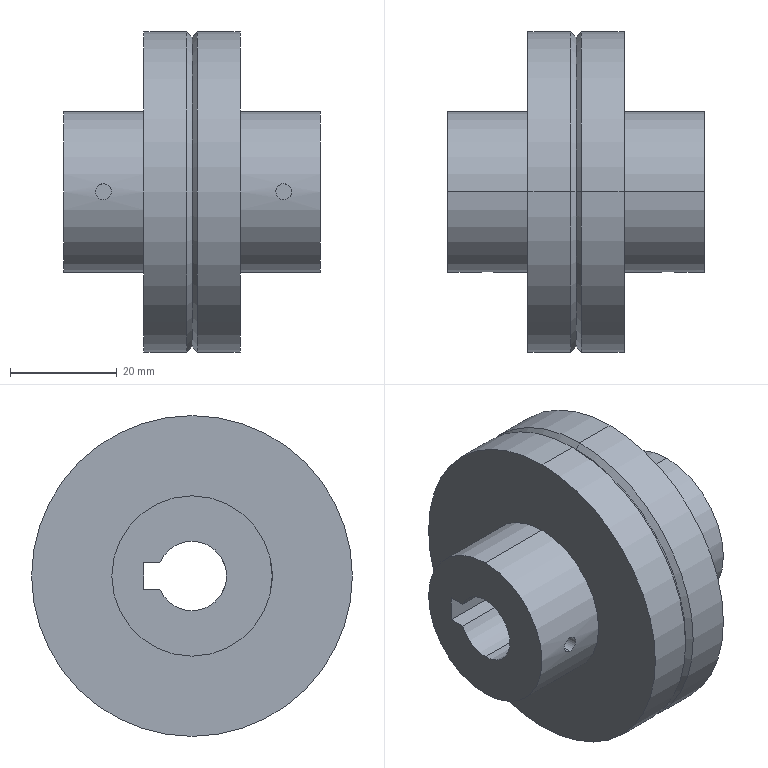Part | NX | features BREP 1 | 1 solid | 32 faces | box 48 x 60 x 60 mm | volume 63736 mm3 | cylinder 18 | plane 10 | cone 4 | commonest cylinder face diameters 3 x4 30 x4 60 x4 13 x3 15 x3
STEP:
#1=CARTESIAN_POINT('',(7.432,-6.331,-1.474));
#2=VERTEX_POINT('',#1);
#3=CARTESIAN_POINT('',(7.432,-6.318,1.526));
#4=VERTEX_POINT('',#3);
#5=CARTESIAN_POINT('',(7.432,-6.331,-1.474));
#6=CARTESIAN_POINT('',(7.034,-6.331,-1.474));
#7=CARTESIAN_POINT('',(6.259,-6.418,-1.149));
#8=CARTESIAN_POINT('',(5.768,-6.543,0.02457));
#9=CARTESIAN_POINT('',(6.259,-6.409,1.201));
#10=CARTESIAN_POINT('',(7.034,-6.318,1.526));
#11=CARTESIAN_POINT('',(7.432,-6.318,1.526));
#12=B_SPLINE_CURVE_WITH_KNOTS('',3,(#5,#6,#7,#8,#9,#10,#11),.UNSPECIFIED.,.F.,.F.,(4,1,1,1,4),(0.,0.001176,0.002352,0.003528,0.004704),.UNSPECIFIED.);
#13=EDGE_CURVE('',#2,#4,#12,.T.);
#14=ORIENTED_EDGE('',*,*,#13,.T.);
#15=CARTESIAN_POINT('',(7.432,-14.919,1.561));
#16=VERTEX_POINT('',#15);
#17=CARTESIAN_POINT('',(7.432,-14.994,1.561));
#18=DIRECTION('',(0.,-1.,0.004061));
#19=VECTOR('',#18,1000.);
#20=LINE('',#17,#19);
#21=EDGE_CURVE('',#16,#4,#20,.F.);
#22=ORIENTED_EDGE('',*,*,#21,.F.);
#23=CARTESIAN_POINT('',(7.432,-14.931,-1.439));
#24=VERTEX_POINT('',#23);
#25=CARTESIAN_POINT('',(7.432,-14.919,1.561));
#26=CARTESIAN_POINT('',(7.035,-14.919,1.561));
#27=CARTESIAN_POINT('',(6.259,-14.958,1.236));
#28=CARTESIAN_POINT('',(5.769,-15.019,0.0625));
#29=CARTESIAN_POINT('',(6.258,-14.967,-1.114));
#30=CARTESIAN_POINT('',(7.035,-14.931,-1.439));
#31=CARTESIAN_POINT('',(7.432,-14.931,-1.439));
#32=B_SPLINE_CURVE_WITH_KNOTS('',3,(#25,#26,#27,#28,#29,#30,#31),.UNSPECIFIED.,.F.,.F.,(4,1,1,1,4),(0.,0.001173,0.002346,0.003519,0.004692),.UNSPECIFIED.);
#33=EDGE_CURVE('',#16,#24,#32,.T.);
#34=ORIENTED_EDGE('',*,*,#33,.T.);
#35=CARTESIAN_POINT('',(7.432,-15.006,-1.439));
#36=DIRECTION('',(0.,-1.,0.004061));
#37=VECTOR('',#36,1000.);
#38=LINE('',#35,#37);
#39=EDGE_CURVE('',#24,#2,#38,.F.);
#40=ORIENTED_EDGE('',*,*,#39,.T.);
#41=EDGE_LOOP('',(#14,#22,#34,#40));
#42=FACE_BOUND('',#41,.T.);
#43=CARTESIAN_POINT('',(7.432,-15.,0.06091));
#44=DIRECTION('',(0.,-1.,0.004061));
#45=DIRECTION('',(0.,0.004061,1.));
#46=AXIS2_PLACEMENT_3D('',#43,#44,#45);
#47=CYLINDRICAL_SURFACE('',#46,1.5);
#48=ADVANCED_FACE('',(#42),#47,.F.);
#49=CARTESIAN_POINT('',(41.177,-7.354,-1.47));
#50=VERTEX_POINT('',#49);
#51=CARTESIAN_POINT('',(41.177,-7.342,1.53));
#52=VERTEX_POINT('',#51);
#53=CARTESIAN_POINT('',(41.177,-7.354,-1.47));
#54=CARTESIAN_POINT('',(40.78,-7.354,-1.47));
#55=CARTESIAN_POINT('',(40.004,-7.43,-1.145));
#56=CARTESIAN_POINT('',(39.514,-7.537,0.02875));
#57=CARTESIAN_POINT('',(40.003,-7.42,1.205));
#58=CARTESIAN_POINT('',(40.78,-7.342,1.53));
#59=CARTESIAN_POINT('',(41.177,-7.342,1.53));
#60=B_SPLINE_CURVE_WITH_KNOTS('',3,(#53,#54,#55,#56,#57,#58,#59),.UNSPECIFIED.,.F.,.F.,(4,1,1,1,4),(0.,0.001175,0.00235,0.003525,0.0047),.UNSPECIFIED.);
#61=EDGE_CURVE('',#50,#52,#60,.T.);
#62=ORIENTED_EDGE('',*,*,#61,.T.);
#63=CARTESIAN_POINT('',(41.177,-14.919,1.561));
#64=VERTEX_POINT('',#63);
#65=CARTESIAN_POINT('',(41.177,-14.994,1.561));
#66=DIRECTION('',(0.,-1.,0.004061));
#67=VECTOR('',#66,1000.);
#68=LINE('',#65,#67);
#69=EDGE_CURVE('',#64,#52,#68,.F.);
#70=ORIENTED_EDGE('',*,*,#69,.F.);
#71=CARTESIAN_POINT('',(41.177,-14.931,-1.439));
#72=VERTEX_POINT('',#71);
#73=CARTESIAN_POINT('',(41.177,-14.919,1.561));
#74=CARTESIAN_POINT('',(40.781,-14.919,1.561));
#75=CARTESIAN_POINT('',(40.004,-14.958,1.236));
#76=CARTESIAN_POINT('',(39.514,-15.019,0.0625));
#77=CARTESIAN_POINT('',(40.003,-14.967,-1.114));
#78=CARTESIAN_POINT('',(40.781,-14.931,-1.439));
#79=CARTESIAN_POINT('',(41.177,-14.931,-1.439));
#80=B_SPLINE_CURVE_WITH_KNOTS('',3,(#73,#74,#75,#76,#77,#78,#79),.UNSPECIFIED.,.F.,.F.,(4,1,1,1,4),(0.,0.001173,0.002346,0.003519,0.004692),.UNSPECIFIED.);
#81=EDGE_CURVE('',#64,#72,#80,.T.);
#82=ORIENTED_EDGE('',*,*,#81,.T.);
#83=CARTESIAN_POINT('',(41.177,-15.006,-1.439));
#84=DIRECTION('',(0.,-1.,0.004061));
#85=VECTOR('',#84,1000.);
#86=LINE('',#83,#85);
#87=EDGE_CURVE('',#72,#50,#86,.F.);
#88=ORIENTED_EDGE('',*,*,#87,.T.);
#89=EDGE_LOOP('',(#62,#70,#82,#88));
#90=FACE_BOUND('',#89,.T.);
#91=CARTESIAN_POINT('',(41.177,-15.,0.06091));
#92=DIRECTION('',(0.,-1.,0.004061));
#93=DIRECTION('',(0.,0.004061,1.));
#94=AXIS2_PLACEMENT_3D('',#91,#92,#93);
#95=CYLINDRICAL_SURFACE('',#94,1.5);
#96=ADVANCED_FACE('',(#90),#95,.F.);
#97=CARTESIAN_POINT('',(24.,0.,29.));
#98=VERTEX_POINT('',#97);
#99=CARTESIAN_POINT('',(24.,0.,-29.));
#100=VERTEX_POINT('',#99);
#101=CARTESIAN_POINT('',(24.,0.,0.));
#102=DIRECTION('',(-1.,0.,0.));
#103=DIRECTION('',(0.,0.,1.));
#104=AXIS2_PLACEMENT_3D('',#101,#102,#103);
#105=CIRCLE('',#104,29.);
#106=EDGE_CURVE('',#98,#100,#105,.T.);
#107=ORIENTED_EDGE('',*,*,#106,.F.);
#108=CARTESIAN_POINT('',(25.,0.,30.));
#109=VERTEX_POINT('',#108);
#110=CARTESIAN_POINT('',(24.,0.,29.));
#111=DIRECTION('',(0.7071,0.,0.7071));
#112=VECTOR('',#111,1000.);
#113=LINE('',#110,#112);
#114=EDGE_CURVE('',#109,#98,#113,.F.);
#115=ORIENTED_EDGE('',*,*,#114,.F.);
#116=CARTESIAN_POINT('',(25.,0.,-30.));
#117=VERTEX_POINT('',#116);
#118=CARTESIAN_POINT('',(25.,0.,0.));
#119=DIRECTION('',(-1.,0.,0.));
#120=DIRECTION('',(0.,0.,1.));
#121=AXIS2_PLACEMENT_3D('',#118,#119,#120);
#122=CIRCLE('',#121,30.);
#123=EDGE_CURVE('',#109,#117,#122,.T.);
#124=ORIENTED_EDGE('',*,*,#123,.T.);
#125=CARTESIAN_POINT('',(24.,0.,-29.));
#126=DIRECTION('',(0.7071,0.,-0.7071));
#127=VECTOR('',#126,1000.);
#128=LINE('',#125,#127);
#129=EDGE_CURVE('',#117,#100,#128,.F.);
#130=ORIENTED_EDGE('',*,*,#129,.T.);
#131=EDGE_LOOP('',(#107,#115,#124,#130));
#132=FACE_BOUND('',#131,.T.);
#133=CARTESIAN_POINT('',(24.,0.,0.));
#134=DIRECTION('',(1.,0.,0.));
#135=DIRECTION('',(0.,0.,1.));
#136=AXIS2_PLACEMENT_3D('',#133,#134,#135);
#137=CONICAL_SURFACE('',#136,29.,0.7854);
#138=ADVANCED_FACE('',(#132),#137,.T.);
#139=CARTESIAN_POINT('',(33.,0.,30.));
#140=VERTEX_POINT('',#139);
#141=CARTESIAN_POINT('',(33.,0.,-30.));
#142=VERTEX_POINT('',#141);
#143=CARTESIAN_POINT('',(33.,0.,0.));
#144=DIRECTION('',(-1.,0.,0.));
#145=DIRECTION('',(0.,0.,1.));
#146=AXIS2_PLACEMENT_3D('',#143,#144,#145);
#147=CIRCLE('',#146,30.);
#148=EDGE_CURVE('',#140,#142,#147,.T.);
#149=ORIENTED_EDGE('',*,*,#148,.T.);
#150=CARTESIAN_POINT('',(0.,0.,-30.));
#151=DIRECTION('',(-1.,0.,0.));
#152=VECTOR('',#151,1000.);
#153=LINE('',#150,#152);
#154=EDGE_CURVE('',#142,#117,#153,.T.);
#155=ORIENTED_EDGE('',*,*,#154,.T.);
#156=ORIENTED_EDGE('',*,*,#123,.F.);
#157=CARTESIAN_POINT('',(0.,0.,30.));
#158=DIRECTION('',(-1.,0.,0.));
#159=VECTOR('',#158,1000.);
#160=LINE('',#157,#159);
#161=EDGE_CURVE('',#140,#109,#160,.T.);
#162=ORIENTED_EDGE('',*,*,#161,.F.);
#163=EDGE_LOOP('',(#149,#155,#156,#162));
#164=FACE_BOUND('',#163,.T.);
#165=CARTESIAN_POINT('',(0.,0.,0.));
#166=DIRECTION('',(-1.,0.,0.));
#167=DIRECTION('',(0.,0.,-1.));
#168=AXIS2_PLACEMENT_3D('',#165,#166,#167);
#169=CYLINDRICAL_SURFACE('',#168,30.);
#170=ADVANCED_FACE('',(#164),#169,.T.);
#171=CARTESIAN_POINT('',(48.,0.,15.));
#172=VERTEX_POINT('',#171);
#173=CARTESIAN_POINT('',(48.,0.,-15.));
#174=VERTEX_POINT('',#173);
#175=CARTESIAN_POINT('',(48.,0.,0.));
#176=DIRECTION('',(-1.,0.,0.));
#177=DIRECTION('',(0.,0.,1.));
#178=AXIS2_PLACEMENT_3D('',#175,#176,#177);
#179=CIRCLE('',#178,15.);
#180=EDGE_CURVE('',#172,#174,#179,.T.);
#181=ORIENTED_EDGE('',*,*,#180,.T.);
#182=CARTESIAN_POINT('',(33.,0.,-15.));
#183=VERTEX_POINT('',#182);
#184=CARTESIAN_POINT('',(0.,0.,-15.));
#185=DIRECTION('',(-1.,0.,0.));
#186=VECTOR('',#185,1000.);
#187=LINE('',#184,#186);
#188=EDGE_CURVE('',#174,#183,#187,.T.);
#189=ORIENTED_EDGE('',*,*,#188,.T.);
#190=CARTESIAN_POINT('',(33.,0.,15.));
#191=VERTEX_POINT('',#190);
#192=CARTESIAN_POINT('',(33.,0.,0.));
#193=DIRECTION('',(-1.,0.,0.));
#194=DIRECTION('',(0.,0.,1.));
#195=AXIS2_PLACEMENT_3D('',#192,#193,#194);
#196=CIRCLE('',#195,15.);
#197=EDGE_CURVE('',#191,#183,#196,.T.);
#198=ORIENTED_EDGE('',*,*,#197,.F.);
#199=CARTESIAN_POINT('',(0.,0.,15.));
#200=DIRECTION('',(-1.,0.,0.));
#201=VECTOR('',#200,1000.);
#202=LINE('',#199,#201);
#203=EDGE_CURVE('',#172,#191,#202,.T.);
#204=ORIENTED_EDGE('',*,*,#203,.F.);
#205=EDGE_LOOP('',(#181,#189,#198,#204));
#206=FACE_BOUND('',#205,.T.);
#207=CARTESIAN_POINT('',(0.,0.,0.));
#208=DIRECTION('',(-1.,0.,0.));
#209=DIRECTION('',(0.,0.,-1.));
#210=AXIS2_PLACEMENT_3D('',#207,#208,#209);
#211=CYLINDRICAL_SURFACE('',#210,15.);
#212=ADVANCED_FACE('',(#206),#211,.T.);
#213=CARTESIAN_POINT('',(48.,0.,-7.5));
#214=VERTEX_POINT('',#213);
#215=CARTESIAN_POINT('',(48.,0.,7.5));
#216=VERTEX_POINT('',#215);
#217=CARTESIAN_POINT('',(48.,0.,0.));
#218=DIRECTION('',(-1.,0.,0.));
#219=DIRECTION('',(0.,0.,1.));
#220=AXIS2_PLACEMENT_3D('',#217,#218,#219);
#221=CIRCLE('',#220,7.5);
#222=EDGE_CURVE('',#214,#216,#221,.T.);
#223=ORIENTED_EDGE('',*,*,#222,.F.);
#224=CARTESIAN_POINT('',(24.,0.,-7.5));
#225=VERTEX_POINT('',#224);
#226=CARTESIAN_POINT('',(0.,0.,-7.5));
#227=DIRECTION('',(-1.,0.,0.));
#228=VECTOR('',#227,1000.);
#229=LINE('',#226,#228);
#230=EDGE_CURVE('',#214,#225,#229,.T.);
#231=ORIENTED_EDGE('',*,*,#230,.T.);
#232=CARTESIAN_POINT('',(24.,0.,7.5));
#233=VERTEX_POINT('',#232);
#234=CARTESIAN_POINT('',(24.,0.,0.));
#235=DIRECTION('',(-1.,0.,0.));
#236=DIRECTION('',(0.,0.,1.));
#237=AXIS2_PLACEMENT_3D('',#234,#235,#236);
#238=CIRCLE('',#237,7.5);
#239=EDGE_CURVE('',#225,#233,#238,.T.);
#240=ORIENTED_EDGE('',*,*,#239,.T.);
#241=CARTESIAN_POINT('',(0.,0.,7.5));
#242=DIRECTION('',(-1.,0.,0.));
#243=VECTOR('',#242,1000.);
#244=LINE('',#241,#243);
#245=EDGE_CURVE('',#216,#233,#244,.T.);
#246=ORIENTED_EDGE('',*,*,#245,.F.);
#247=EDGE_LOOP('',(#223,#231,#240,#246));
#248=FACE_BOUND('',#247,.T.);
#249=ORIENTED_EDGE('',*,*,#61,.F.);
#250=CARTESIAN_POINT('',(41.177,-7.342,1.53));
#251=CARTESIAN_POINT('',(41.575,-7.342,1.53));
#252=CARTESIAN_POINT('',(42.35,-7.42,1.205));
#253=CARTESIAN_POINT('',(42.841,-7.537,0.03247));
#254=CARTESIAN_POINT('',(42.351,-7.43,-1.145));
#255=CARTESIAN_POINT('',(41.575,-7.354,-1.47));
#256=CARTESIAN_POINT('',(41.177,-7.354,-1.47));
#257=B_SPLINE_CURVE_WITH_KNOTS('',3,(#250,#251,#252,#253,#254,#255,#256),.UNSPECIFIED.,.F.,.F.,(4,1,1,1,4),(0.,0.001175,0.00235,0.003525,0.0047),.UNSPECIFIED.);
#258=EDGE_CURVE('',#52,#50,#257,.T.);
#259=ORIENTED_EDGE('',*,*,#258,.F.);
#260=EDGE_LOOP('',(#249,#259));
#261=FACE_BOUND('',#260,.T.);
#262=CARTESIAN_POINT('',(0.,0.,0.));
#263=DIRECTION('',(-1.,0.,0.));
#264=DIRECTION('',(0.,0.,-1.));
#265=AXIS2_PLACEMENT_3D('',#262,#263,#264);
#266=CYLINDRICAL_SURFACE('',#265,7.5);
#267=ADVANCED_FACE('',(#248,#261),#266,.F.);
#268=CARTESIAN_POINT('',(48.,7.071,2.5));
#269=VERTEX_POINT('',#268);
#270=CARTESIAN_POINT('',(48.,0.,0.));
#271=DIRECTION('',(-1.,0.,0.));
#272=DIRECTION('',(0.,0.,1.));
#273=AXIS2_PLACEMENT_3D('',#270,#271,#272);
#274=CIRCLE('',#273,7.5);
#275=EDGE_CURVE('',#216,#269,#274,.T.);
#276=ORIENTED_EDGE('',*,*,#275,.F.);
#277=ORIENTED_EDGE('',*,*,#245,.T.);
#278=CARTESIAN_POINT('',(24.,7.071,2.5));
#279=VERTEX_POINT('',#278);
#280=CARTESIAN_POINT('',(24.,0.,0.));
#281=DIRECTION('',(-1.,0.,0.));
#282=DIRECTION('',(0.,0.,1.));
#283=AXIS2_PLACEMENT_3D('',#280,#281,#282);
#284=CIRCLE('',#283,7.5);
#285=EDGE_CURVE('',#233,#279,#284,.T.);
#286=ORIENTED_EDGE('',*,*,#285,.T.);
#287=CARTESIAN_POINT('',(24.,7.071,2.5));
#288=DIRECTION('',(1.,0.,0.));
#289=VECTOR('',#288,1000.);
#290=LINE('',#287,#289);
#291=EDGE_CURVE('',#279,#269,#290,.T.);
#292=ORIENTED_EDGE('',*,*,#291,.T.);
#293=EDGE_LOOP('',(#276,#277,#286,#292));
#294=FACE_BOUND('',#293,.T.);
#295=CARTESIAN_POINT('',(0.,0.,0.));
#296=DIRECTION('',(-1.,0.,0.));
#297=DIRECTION('',(0.,0.,-1.));
#298=AXIS2_PLACEMENT_3D('',#295,#296,#297);
#299=CYLINDRICAL_SURFACE('',#298,7.5);
#300=ADVANCED_FACE('',(#294),#299,.F.);
#301=CARTESIAN_POINT('',(24.,0.,-6.5));
#302=VERTEX_POINT('',#301);
#303=CARTESIAN_POINT('',(24.,0.,6.5));
#304=VERTEX_POINT('',#303);
#305=CARTESIAN_POINT('',(24.,0.,0.));
#306=DIRECTION('',(-1.,0.,0.));
#307=DIRECTION('',(0.,0.,1.));
#308=AXIS2_PLACEMENT_3D('',#305,#306,#307);
#309=CIRCLE('',#308,6.5);
#310=EDGE_CURVE('',#302,#304,#309,.T.);
#311=ORIENTED_EDGE('',*,*,#310,.F.);
#312=CARTESIAN_POINT('',(0.,0.,-6.5));
#313=VERTEX_POINT('',#312);
#314=CARTESIAN_POINT('',(0.,0.,-6.5));
#315=DIRECTION('',(-1.,0.,0.));
#316=VECTOR('',#315,1000.);
#317=LINE('',#314,#316);
#318=EDGE_CURVE('',#302,#313,#317,.T.);
#319=ORIENTED_EDGE('',*,*,#318,.T.);
#320=CARTESIAN_POINT('',(0.,0.,6.5));
#321=VERTEX_POINT('',#320);
#322=CARTESIAN_POINT('',(0.,0.,0.));
#323=DIRECTION('',(-1.,0.,0.));
#324=DIRECTION('',(0.,0.,1.));
#325=AXIS2_PLACEMENT_3D('',#322,#323,#324);
#326=CIRCLE('',#325,6.5);
#327=EDGE_CURVE('',#313,#321,#326,.T.);
#328=ORIENTED_EDGE('',*,*,#327,.T.);
#329=CARTESIAN_POINT('',(0.,0.,6.5));
#330=DIRECTION('',(-1.,0.,0.));
#331=VECTOR('',#330,1000.);
#332=LINE('',#329,#331);
#333=EDGE_CURVE('',#304,#321,#332,.T.);
#334=ORIENTED_EDGE('',*,*,#333,.F.);
#335=EDGE_LOOP('',(#311,#319,#328,#334));
#336=FACE_BOUND('',#335,.T.);
#337=ORIENTED_EDGE('',*,*,#13,.F.);
#338=CARTESIAN_POINT('',(7.432,-6.318,1.526));
#339=CARTESIAN_POINT('',(7.83,-6.318,1.526));
#340=CARTESIAN_POINT('',(8.604,-6.409,1.201));
#341=CARTESIAN_POINT('',(9.096,-6.543,0.02857));
#342=CARTESIAN_POINT('',(8.605,-6.418,-1.149));
#343=CARTESIAN_POINT('',(7.83,-6.331,-1.474));
#344=CARTESIAN_POINT('',(7.432,-6.331,-1.474));
#345=B_SPLINE_CURVE_WITH_KNOTS('',3,(#338,#339,#340,#341,#342,#343,#344),.UNSPECIFIED.,.F.,.F.,(4,1,1,1,4),(0.,0.001176,0.002352,0.003528,0.004704),.UNSPECIFIED.);
#346=EDGE_CURVE('',#4,#2,#345,.T.);
#347=ORIENTED_EDGE('',*,*,#346,.F.);
#348=EDGE_LOOP('',(#337,#347));
#349=FACE_BOUND('',#348,.T.);
#350=CARTESIAN_POINT('',(0.,0.,0.));
#351=DIRECTION('',(-1.,0.,0.));
#352=DIRECTION('',(0.,0.,-1.));
#353=AXIS2_PLACEMENT_3D('',#350,#351,#352);
#354=CYLINDRICAL_SURFACE('',#353,6.5);
#355=ADVANCED_FACE('',(#336,#349),#354,.F.);
#356=CARTESIAN_POINT('',(24.,6.,2.5));
#357=VERTEX_POINT('',#356);
#358=CARTESIAN_POINT('',(24.,0.,0.));
#359=DIRECTION('',(-1.,0.,0.));
#360=DIRECTION('',(0.,0.,1.));
#361=AXIS2_PLACEMENT_3D('',#358,#359,#360);
#362=CIRCLE('',#361,6.5);
#363=EDGE_CURVE('',#304,#357,#362,.T.);
#364=ORIENTED_EDGE('',*,*,#363,.F.);
#365=ORIENTED_EDGE('',*,*,#333,.T.);
#366=CARTESIAN_POINT('',(0.,6.,2.5));
#367=VERTEX_POINT('',#366);
#368=CARTESIAN_POINT('',(0.,0.,0.));
#369=DIRECTION('',(-1.,0.,0.));
#370=DIRECTION('',(0.,0.,1.));
#371=AXIS2_PLACEMENT_3D('',#368,#369,#370);
#372=CIRCLE('',#371,6.5);
#373=EDGE_CURVE('',#321,#367,#372,.T.);
#374=ORIENTED_EDGE('',*,*,#373,.T.);
#375=CARTESIAN_POINT('',(24.,6.,2.5));
#376=DIRECTION('',(-1.,0.,0.));
#377=VECTOR('',#376,1000.);
#378=LINE('',#375,#377);
#379=EDGE_CURVE('',#357,#367,#378,.T.);
#380=ORIENTED_EDGE('',*,*,#379,.F.);
#381=EDGE_LOOP('',(#364,#365,#374,#380));
#382=FACE_BOUND('',#381,.T.);
#383=CARTESIAN_POINT('',(0.,0.,0.));
#384=DIRECTION('',(-1.,0.,0.));
#385=DIRECTION('',(0.,0.,-1.));
#386=AXIS2_PLACEMENT_3D('',#383,#384,#385);
#387=CYLINDRICAL_SURFACE('',#386,6.5);
#388=ADVANCED_FACE('',(#382),#387,.F.);
#389=CARTESIAN_POINT('',(15.,0.,15.));
#390=VERTEX_POINT('',#389);
#391=CARTESIAN_POINT('',(15.,0.,-15.));
#392=VERTEX_POINT('',#391);
#393=CARTESIAN_POINT('',(15.,0.,0.));
#394=DIRECTION('',(-1.,0.,0.));
#395=DIRECTION('',(0.,0.,1.));
#396=AXIS2_PLACEMENT_3D('',#393,#394,#395);
#397=CIRCLE('',#396,15.);
#398=EDGE_CURVE('',#390,#392,#397,.T.);
#399=ORIENTED_EDGE('',*,*,#398,.T.);
#400=CARTESIAN_POINT('',(0.,0.,-15.));
#401=VERTEX_POINT('',#400);
#402=CARTESIAN_POINT('',(0.,0.,-15.));
#403=DIRECTION('',(-1.,0.,0.));
#404=VECTOR('',#403,1000.);
#405=LINE('',#402,#404);
#406=EDGE_CURVE('',#392,#401,#405,.T.);
#407=ORIENTED_EDGE('',*,*,#406,.T.);
#408=CARTESIAN_POINT('',(0.,0.,15.));
#409=VERTEX_POINT('',#408);
#410=CARTESIAN_POINT('',(0.,0.,0.));
#411=DIRECTION('',(-1.,0.,0.));
#412=DIRECTION('',(0.,0.,1.));
#413=AXIS2_PLACEMENT_3D('',#410,#411,#412);
#414=CIRCLE('',#413,15.);
#415=EDGE_CURVE('',#409,#401,#414,.T.);
#416=ORIENTED_EDGE('',*,*,#415,.F.);
#417=CARTESIAN_POINT('',(0.,0.,15.));
#418=DIRECTION('',(-1.,0.,0.));
#419=VECTOR('',#418,1000.);
#420=LINE('',#417,#419);
#421=EDGE_CURVE('',#390,#409,#420,.T.);
#422=ORIENTED_EDGE('',*,*,#421,.F.);
#423=EDGE_LOOP('',(#399,#407,#416,#422));
#424=FACE_BOUND('',#423,.T.);
#425=CARTESIAN_POINT('',(0.,0.,0.));
#426=DIRECTION('',(-1.,0.,0.));
#427=DIRECTION('',(0.,0.,-1.));
#428=AXIS2_PLACEMENT_3D('',#425,#426,#427);
#429=CYLINDRICAL_SURFACE('',#428,15.);
#430=ADVANCED_FACE('',(#424),#429,.T.);
#431=CARTESIAN_POINT('',(23.,0.,30.));
#432=VERTEX_POINT('',#431);
#433=CARTESIAN_POINT('',(23.,0.,-30.));
#434=VERTEX_POINT('',#433);
#435=CARTESIAN_POINT('',(23.,0.,0.));
#436=DIRECTION('',(-1.,0.,0.));
#437=DIRECTION('',(0.,0.,1.));
#438=AXIS2_PLACEMENT_3D('',#435,#436,#437);
#439=CIRCLE('',#438,30.);
#440=EDGE_CURVE('',#432,#434,#439,.T.);
#441=ORIENTED_EDGE('',*,*,#440,.T.);
#442=CARTESIAN_POINT('',(15.,0.,-30.));
#443=VERTEX_POINT('',#442);
#444=CARTESIAN_POINT('',(0.,0.,-30.));
#445=DIRECTION('',(-1.,0.,0.));
#446=VECTOR('',#445,1000.);
#447=LINE('',#444,#446);
#448=EDGE_CURVE('',#434,#443,#447,.T.);
#449=ORIENTED_EDGE('',*,*,#448,.T.);
#450=CARTESIAN_POINT('',(15.,0.,30.));
#451=VERTEX_POINT('',#450);
#452=CARTESIAN_POINT('',(15.,0.,0.));
#453=DIRECTION('',(-1.,0.,0.));
#454=DIRECTION('',(0.,0.,1.));
#455=AXIS2_PLACEMENT_3D('',#452,#453,#454);
#456=CIRCLE('',#455,30.);
#457=EDGE_CURVE('',#451,#443,#456,.T.);
#458=ORIENTED_EDGE('',*,*,#457,.F.);
#459=CARTESIAN_POINT('',(0.,0.,30.));
#460=DIRECTION('',(-1.,0.,0.));
#461=VECTOR('',#460,1000.);
#462=LINE('',#459,#461);
#463=EDGE_CURVE('',#432,#451,#462,.T.);
#464=ORIENTED_EDGE('',*,*,#463,.F.);
#465=EDGE_LOOP('',(#441,#449,#458,#464));
#466=FACE_BOUND('',#465,.T.);
#467=CARTESIAN_POINT('',(0.,0.,0.));
#468=DIRECTION('',(-1.,0.,0.));
#469=DIRECTION('',(0.,0.,-1.));
#470=AXIS2_PLACEMENT_3D('',#467,#468,#469);
#471=CYLINDRICAL_SURFACE('',#470,30.);
#472=ADVANCED_FACE('',(#466),#471,.T.);
#473=ORIENTED_EDGE('',*,*,#106,.T.);
#474=CARTESIAN_POINT('',(23.,0.,-30.));
#475=DIRECTION('',(-0.7071,0.,-0.7071));
#476=VECTOR('',#475,1000.);
#477=LINE('',#474,#476);
#478=EDGE_CURVE('',#100,#434,#477,.T.);
#479=ORIENTED_EDGE('',*,*,#478,.T.);
#480=ORIENTED_EDGE('',*,*,#440,.F.);
#481=CARTESIAN_POINT('',(23.,0.,30.));
#482=DIRECTION('',(-0.7071,0.,0.7071));
#483=VECTOR('',#482,1000.);
#484=LINE('',#481,#483);
#485=EDGE_CURVE('',#98,#432,#484,.T.);
#486=ORIENTED_EDGE('',*,*,#485,.F.);
#487=EDGE_LOOP('',(#473,#479,#480,#486));
#488=FACE_BOUND('',#487,.T.);
#489=CARTESIAN_POINT('',(23.,0.,0.));
#490=DIRECTION('',(-1.,0.,0.));
#491=DIRECTION('',(0.,0.,-1.));
#492=AXIS2_PLACEMENT_3D('',#489,#490,#491);
#493=CONICAL_SURFACE('',#492,30.,0.7854);
#494=ADVANCED_FACE('',(#488),#493,.T.);
#495=CARTESIAN_POINT('',(24.,9.,2.5));
#496=VERTEX_POINT('',#495);
#497=CARTESIAN_POINT('',(24.,9.,-2.5));
#498=VERTEX_POINT('',#497);
#499=CARTESIAN_POINT('',(24.,9.,-2.5));
#500=DIRECTION('',(0.,0.,-1.));
#501=VECTOR('',#500,1000.);
#502=LINE('',#499,#501);
#503=EDGE_CURVE('',#496,#498,#502,.T.);
#504=ORIENTED_EDGE('',*,*,#503,.T.);
#505=CARTESIAN_POINT('',(24.,10.,-2.5));
#506=VERTEX_POINT('',#505);
#507=CARTESIAN_POINT('',(24.,7.071,-2.5));
#508=DIRECTION('',(0.,1.,0.));
#509=VECTOR('',#508,1000.);
#510=LINE('',#507,#509);
#511=EDGE_CURVE('',#498,#506,#510,.T.);
#512=ORIENTED_EDGE('',*,*,#511,.T.);
#513=CARTESIAN_POINT('',(24.,10.,2.5));
#514=VERTEX_POINT('',#513);
#515=CARTESIAN_POINT('',(24.,10.,2.5));
#516=DIRECTION('',(0.,0.,1.));
#517=VECTOR('',#516,1000.);
#518=LINE('',#515,#517);
#519=EDGE_CURVE('',#506,#514,#518,.T.);
#520=ORIENTED_EDGE('',*,*,#519,.T.);
#521=CARTESIAN_POINT('',(24.,7.071,2.5));
#522=DIRECTION('',(0.,-1.,0.));
#523=VECTOR('',#522,1000.);
#524=LINE('',#521,#523);
#525=EDGE_CURVE('',#514,#496,#524,.T.);
#526=ORIENTED_EDGE('',*,*,#525,.T.);
#527=EDGE_LOOP('',(#504,#512,#520,#526));
#528=FACE_BOUND('',#527,.T.);
#529=CARTESIAN_POINT('',(24.,0.,0.));
#530=DIRECTION('',(1.,0.,0.));
#531=DIRECTION('',(0.,-1.,0.));
#532=AXIS2_PLACEMENT_3D('',#529,#530,#531);
#533=PLANE('',#532);
#534=ADVANCED_FACE('',(#528),#533,.T.);
#535=ORIENTED_EDGE('',*,*,#478,.F.);
#536=CARTESIAN_POINT('',(24.,0.,0.));
#537=DIRECTION('',(-1.,0.,0.));
#538=DIRECTION('',(0.,0.,1.));
#539=AXIS2_PLACEMENT_3D('',#536,#537,#538);
#540=CIRCLE('',#539,29.);
#541=EDGE_CURVE('',#100,#98,#540,.T.);
#542=ORIENTED_EDGE('',*,*,#541,.T.);
#543=ORIENTED_EDGE('',*,*,#485,.T.);
#544=CARTESIAN_POINT('',(23.,0.,0.));
#545=DIRECTION('',(-1.,0.,0.));
#546=DIRECTION('',(0.,0.,1.));
#547=AXIS2_PLACEMENT_3D('',#544,#545,#546);
#548=CIRCLE('',#547,30.);
#549=EDGE_CURVE('',#434,#432,#548,.T.);
#550=ORIENTED_EDGE('',*,*,#549,.F.);
#551=EDGE_LOOP('',(#535,#542,#543,#550));
#552=FACE_BOUND('',#551,.T.);
#553=CARTESIAN_POINT('',(23.,0.,0.));
#554=DIRECTION('',(-1.,0.,0.));
#555=DIRECTION('',(0.,0.,-1.));
#556=AXIS2_PLACEMENT_3D('',#553,#554,#555);
#557=CONICAL_SURFACE('',#556,30.,0.7854);
#558=ADVANCED_FACE('',(#552),#557,.T.);
#559=ORIENTED_EDGE('',*,*,#448,.F.);
#560=ORIENTED_EDGE('',*,*,#549,.T.);
#561=ORIENTED_EDGE('',*,*,#463,.T.);
#562=CARTESIAN_POINT('',(15.,0.,0.));
#563=DIRECTION('',(-1.,0.,0.));
#564=DIRECTION('',(0.,0.,1.));
#565=AXIS2_PLACEMENT_3D('',#562,#563,#564);
#566=CIRCLE('',#565,30.);
#567=EDGE_CURVE('',#443,#451,#566,.T.);
#568=ORIENTED_EDGE('',*,*,#567,.F.);
#569=EDGE_LOOP('',(#559,#560,#561,#568));
#570=FACE_BOUND('',#569,.T.);
#571=CARTESIAN_POINT('',(0.,0.,0.));
#572=DIRECTION('',(-1.,0.,0.));
#573=DIRECTION('',(0.,0.,-1.));
#574=AXIS2_PLACEMENT_3D('',#571,#572,#573);
#575=CYLINDRICAL_SURFACE('',#574,30.);
#576=ADVANCED_FACE('',(#570),#575,.T.);
#577=ORIENTED_EDGE('',*,*,#457,.T.);
#578=ORIENTED_EDGE('',*,*,#567,.T.);
#579=EDGE_LOOP('',(#577,#578));
#580=FACE_BOUND('',#579,.T.);
#581=ORIENTED_EDGE('',*,*,#398,.F.);
#582=CARTESIAN_POINT('',(15.,0.,0.));
#583=DIRECTION('',(-1.,0.,0.));
#584=DIRECTION('',(0.,0.,1.));
#585=AXIS2_PLACEMENT_3D('',#582,#583,#584);
#586=CIRCLE('',#585,15.);
#587=EDGE_CURVE('',#392,#390,#586,.T.);
#588=ORIENTED_EDGE('',*,*,#587,.F.);
#589=EDGE_LOOP('',(#581,#588));
#590=FACE_BOUND('',#589,.T.);
#591=CARTESIAN_POINT('',(15.,0.,0.));
#592=DIRECTION('',(-1.,0.,0.));
#593=DIRECTION('',(0.,-1.,0.));
#594=AXIS2_PLACEMENT_3D('',#591,#592,#593);
#595=PLANE('',#594);
#596=ADVANCED_FACE('',(#580,#590),#595,.T.);
#597=ORIENTED_EDGE('',*,*,#406,.F.);
#598=ORIENTED_EDGE('',*,*,#587,.T.);
#599=ORIENTED_EDGE('',*,*,#421,.T.);
#600=CARTESIAN_POINT('',(0.,0.,0.));
#601=DIRECTION('',(-1.,0.,0.));
#602=DIRECTION('',(0.,0.,1.));
#603=AXIS2_PLACEMENT_3D('',#600,#601,#602);
#604=CIRCLE('',#603,15.);
#605=EDGE_CURVE('',#401,#409,#604,.T.);
#606=ORIENTED_EDGE('',*,*,#605,.F.);
#607=EDGE_LOOP('',(#597,#598,#599,#606));
#608=FACE_BOUND('',#607,.T.);
#609=CARTESIAN_POINT('',(7.432,-14.931,-1.439));
#610=CARTESIAN_POINT('',(7.829,-14.931,-1.439));
#611=CARTESIAN_POINT('',(8.605,-14.967,-1.114));
#612=CARTESIAN_POINT('',(9.095,-15.019,0.05948));
#613=CARTESIAN_POINT('',(8.606,-14.958,1.235));
#614=CARTESIAN_POINT('',(7.829,-14.919,1.561));
#615=CARTESIAN_POINT('',(7.432,-14.919,1.561));
#616=B_SPLINE_CURVE_WITH_KNOTS('',3,(#609,#610,#611,#612,#613,#614,#615),.UNSPECIFIED.,.F.,.F.,(4,1,1,1,4),(0.,0.001173,0.002346,0.003519,0.004692),.UNSPECIFIED.);
#617=EDGE_CURVE('',#24,#16,#616,.T.);
#618=ORIENTED_EDGE('',*,*,#617,.F.);
#619=ORIENTED_EDGE('',*,*,#33,.F.);
#620=EDGE_LOOP('',(#618,#619));
#621=FACE_BOUND('',#620,.T.);
#622=CARTESIAN_POINT('',(0.,0.,0.));
#623=DIRECTION('',(-1.,0.,0.));
#624=DIRECTION('',(0.,0.,-1.));
#625=AXIS2_PLACEMENT_3D('',#622,#623,#624);
#626=CYLINDRICAL_SURFACE('',#625,15.);
#627=ADVANCED_FACE('',(#608,#621),#626,.T.);
#628=ORIENTED_EDGE('',*,*,#415,.T.);
#629=ORIENTED_EDGE('',*,*,#605,.T.);
#630=EDGE_LOOP('',(#628,#629));
#631=FACE_BOUND('',#630,.T.);
#632=CARTESIAN_POINT('',(0.,9.,2.5));
#633=VERTEX_POINT('',#632);
#634=CARTESIAN_POINT('',(0.,6.,2.5));
#635=DIRECTION('',(0.,1.,0.));
#636=VECTOR('',#635,1000.);
#637=LINE('',#634,#636);
#638=EDGE_CURVE('',#367,#633,#637,.T.);
#639=ORIENTED_EDGE('',*,*,#638,.F.);
#640=ORIENTED_EDGE('',*,*,#373,.F.);
#641=ORIENTED_EDGE('',*,*,#327,.F.);
#642=CARTESIAN_POINT('',(0.,6.,-2.5));
#643=VERTEX_POINT('',#642);
#644=CARTESIAN_POINT('',(0.,0.,0.));
#645=DIRECTION('',(-1.,0.,0.));
#646=DIRECTION('',(0.,0.,1.));
#647=AXIS2_PLACEMENT_3D('',#644,#645,#646);
#648=CIRCLE('',#647,6.5);
#649=EDGE_CURVE('',#643,#313,#648,.T.);
#650=ORIENTED_EDGE('',*,*,#649,.F.);
#651=CARTESIAN_POINT('',(0.,9.,-2.5));
#652=VERTEX_POINT('',#651);
#653=CARTESIAN_POINT('',(0.,6.,-2.5));
#654=DIRECTION('',(0.,-1.,0.));
#655=VECTOR('',#654,1000.);
#656=LINE('',#653,#655);
#657=EDGE_CURVE('',#652,#643,#656,.T.);
#658=ORIENTED_EDGE('',*,*,#657,.F.);
#659=CARTESIAN_POINT('',(0.,9.,-2.5));
#660=DIRECTION('',(0.,0.,-1.));
#661=VECTOR('',#660,1000.);
#662=LINE('',#659,#661);
#663=EDGE_CURVE('',#633,#652,#662,.T.);
#664=ORIENTED_EDGE('',*,*,#663,.F.);
#665=EDGE_LOOP('',(#639,#640,#641,#650,#658,#664));
#666=FACE_BOUND('',#665,.T.);
#667=CARTESIAN_POINT('',(0.,0.,0.));
#668=DIRECTION('',(-1.,0.,0.));
#669=DIRECTION('',(0.,-1.,0.));
#670=AXIS2_PLACEMENT_3D('',#667,#668,#669);
#671=PLANE('',#670);
#672=ADVANCED_FACE('',(#631,#666),#671,.T.);
#673=ORIENTED_EDGE('',*,*,#318,.F.);
#674=CARTESIAN_POINT('',(24.,6.,-2.5));
#675=VERTEX_POINT('',#674);
#676=CARTESIAN_POINT('',(24.,0.,0.));
#677=DIRECTION('',(-1.,0.,0.));
#678=DIRECTION('',(0.,0.,1.));
#679=AXIS2_PLACEMENT_3D('',#676,#677,#678);
#680=CIRCLE('',#679,6.5);
#681=EDGE_CURVE('',#675,#302,#680,.T.);
#682=ORIENTED_EDGE('',*,*,#681,.F.);
#683=CARTESIAN_POINT('',(24.,6.,-2.5));
#684=DIRECTION('',(-1.,0.,0.));
#685=VECTOR('',#684,1000.);
#686=LINE('',#683,#685);
#687=EDGE_CURVE('',#675,#643,#686,.T.);
#688=ORIENTED_EDGE('',*,*,#687,.T.);
#689=ORIENTED_EDGE('',*,*,#649,.T.);
#690=EDGE_LOOP('',(#673,#682,#688,#689));
#691=FACE_BOUND('',#690,.T.);
#692=CARTESIAN_POINT('',(0.,0.,0.));
#693=DIRECTION('',(-1.,0.,0.));
#694=DIRECTION('',(0.,0.,-1.));
#695=AXIS2_PLACEMENT_3D('',#692,#693,#694);
#696=CYLINDRICAL_SURFACE('',#695,6.5);
#697=ADVANCED_FACE('',(#691),#696,.F.);
#698=CARTESIAN_POINT('',(24.,6.,2.5));
#699=DIRECTION('',(0.,1.,0.));
#700=VECTOR('',#699,1000.);
#701=LINE('',#698,#700);
#702=EDGE_CURVE('',#357,#279,#701,.T.);
#703=ORIENTED_EDGE('',*,*,#702,.T.);
#704=ORIENTED_EDGE('',*,*,#285,.F.);
#705=ORIENTED_EDGE('',*,*,#239,.F.);
#706=CARTESIAN_POINT('',(24.,7.071,-2.5));
#707=VERTEX_POINT('',#706);
#708=CARTESIAN_POINT('',(24.,0.,0.));
#709=DIRECTION('',(-1.,0.,0.));
#710=DIRECTION('',(0.,0.,1.));
#711=AXIS2_PLACEMENT_3D('',#708,#709,#710);
#712=CIRCLE('',#711,7.5);
#713=EDGE_CURVE('',#707,#225,#712,.T.);
#714=ORIENTED_EDGE('',*,*,#713,.F.);
#715=CARTESIAN_POINT('',(24.,6.,-2.5));
#716=DIRECTION('',(0.,-1.,0.));
#717=VECTOR('',#716,1000.);
#718=LINE('',#715,#717);
#719=EDGE_CURVE('',#707,#675,#718,.T.);
#720=ORIENTED_EDGE('',*,*,#719,.T.);
#721=ORIENTED_EDGE('',*,*,#681,.T.);
#722=ORIENTED_EDGE('',*,*,#310,.T.);
#723=ORIENTED_EDGE('',*,*,#363,.T.);
#724=EDGE_LOOP('',(#703,#704,#705,#714,#720,#721,#722,#723));
#725=FACE_BOUND('',#724,.T.);
#726=CARTESIAN_POINT('',(24.,0.,0.));
#727=DIRECTION('',(1.,0.,0.));
#728=DIRECTION('',(0.,-1.,0.));
#729=AXIS2_PLACEMENT_3D('',#726,#727,#728);
#730=PLANE('',#729);
#731=ADVANCED_FACE('',(#725),#730,.T.);
#732=ORIENTED_EDGE('',*,*,#230,.F.);
#733=CARTESIAN_POINT('',(48.,7.071,-2.5));
#734=VERTEX_POINT('',#733);
#735=CARTESIAN_POINT('',(48.,0.,0.));
#736=DIRECTION('',(-1.,0.,0.));
#737=DIRECTION('',(0.,0.,1.));
#738=AXIS2_PLACEMENT_3D('',#735,#736,#737);
#739=CIRCLE('',#738,7.5);
#740=EDGE_CURVE('',#734,#214,#739,.T.);
#741=ORIENTED_EDGE('',*,*,#740,.F.);
#742=CARTESIAN_POINT('',(24.,7.071,-2.5));
#743=DIRECTION('',(1.,0.,0.));
#744=VECTOR('',#743,1000.);
#745=LINE('',#742,#744);
#746=EDGE_CURVE('',#707,#734,#745,.T.);
#747=ORIENTED_EDGE('',*,*,#746,.F.);
#748=ORIENTED_EDGE('',*,*,#713,.T.);
#749=EDGE_LOOP('',(#732,#741,#747,#748));
#750=FACE_BOUND('',#749,.T.);
#751=CARTESIAN_POINT('',(0.,0.,0.));
#752=DIRECTION('',(-1.,0.,0.));
#753=DIRECTION('',(0.,0.,-1.));
#754=AXIS2_PLACEMENT_3D('',#751,#752,#753);
#755=CYLINDRICAL_SURFACE('',#754,7.5);
#756=ADVANCED_FACE('',(#750),#755,.F.);
#757=ORIENTED_EDGE('',*,*,#180,.F.);
#758=CARTESIAN_POINT('',(48.,0.,0.));
#759=DIRECTION('',(-1.,0.,0.));
#760=DIRECTION('',(0.,0.,1.));
#761=AXIS2_PLACEMENT_3D('',#758,#759,#760);
#762=CIRCLE('',#761,15.);
#763=EDGE_CURVE('',#174,#172,#762,.T.);
#764=ORIENTED_EDGE('',*,*,#763,.F.);
#765=EDGE_LOOP('',(#757,#764));
#766=FACE_BOUND('',#765,.T.);
#767=CARTESIAN_POINT('',(48.,10.,-2.5));
#768=VERTEX_POINT('',#767);
#769=CARTESIAN_POINT('',(48.,7.071,-2.5));
#770=DIRECTION('',(0.,1.,0.));
#771=VECTOR('',#770,1000.);
#772=LINE('',#769,#771);
#773=EDGE_CURVE('',#734,#768,#772,.T.);
#774=ORIENTED_EDGE('',*,*,#773,.F.);
#775=ORIENTED_EDGE('',*,*,#740,.T.);
#776=ORIENTED_EDGE('',*,*,#222,.T.);
#777=ORIENTED_EDGE('',*,*,#275,.T.);
#778=CARTESIAN_POINT('',(48.,10.,2.5));
#779=VERTEX_POINT('',#778);
#780=CARTESIAN_POINT('',(48.,7.071,2.5));
#781=DIRECTION('',(0.,-1.,0.));
#782=VECTOR('',#781,1000.);
#783=LINE('',#780,#782);
#784=EDGE_CURVE('',#779,#269,#783,.T.);
#785=ORIENTED_EDGE('',*,*,#784,.F.);
#786=CARTESIAN_POINT('',(48.,10.,2.5));
#787=DIRECTION('',(0.,0.,1.));
#788=VECTOR('',#787,1000.);
#789=LINE('',#786,#788);
#790=EDGE_CURVE('',#768,#779,#789,.T.);
#791=ORIENTED_EDGE('',*,*,#790,.F.);
#792=EDGE_LOOP('',(#774,#775,#776,#777,#785,#791));
#793=FACE_BOUND('',#792,.T.);
#794=CARTESIAN_POINT('',(48.,0.,0.));
#795=DIRECTION('',(1.,0.,0.));
#796=DIRECTION('',(0.,-1.,0.));
#797=AXIS2_PLACEMENT_3D('',#794,#795,#796);
#798=PLANE('',#797);
#799=ADVANCED_FACE('',(#766,#793),#798,.T.);
#800=ORIENTED_EDGE('',*,*,#188,.F.);
#801=ORIENTED_EDGE('',*,*,#763,.T.);
#802=ORIENTED_EDGE('',*,*,#203,.T.);
#803=CARTESIAN_POINT('',(33.,0.,0.));
#804=DIRECTION('',(-1.,0.,0.));
#805=DIRECTION('',(0.,0.,1.));
#806=AXIS2_PLACEMENT_3D('',#803,#804,#805);
#807=CIRCLE('',#806,15.);
#808=EDGE_CURVE('',#183,#191,#807,.T.);
#809=ORIENTED_EDGE('',*,*,#808,.F.);
#810=EDGE_LOOP('',(#800,#801,#802,#809));
#811=FACE_BOUND('',#810,.T.);
#812=CARTESIAN_POINT('',(41.177,-14.931,-1.439));
#813=CARTESIAN_POINT('',(41.574,-14.931,-1.439));
#814=CARTESIAN_POINT('',(42.35,-14.967,-1.114));
#815=CARTESIAN_POINT('',(42.84,-15.019,0.05948));
#816=CARTESIAN_POINT('',(42.351,-14.958,1.235));
#817=CARTESIAN_POINT('',(41.574,-14.919,1.561));
#818=CARTESIAN_POINT('',(41.177,-14.919,1.561));
#819=B_SPLINE_CURVE_WITH_KNOTS('',3,(#812,#813,#814,#815,#816,#817,#818),.UNSPECIFIED.,.F.,.F.,(4,1,1,1,4),(0.,0.001173,0.002346,0.003519,0.004692),.UNSPECIFIED.);
#820=EDGE_CURVE('',#72,#64,#819,.T.);
#821=ORIENTED_EDGE('',*,*,#820,.F.);
#822=ORIENTED_EDGE('',*,*,#81,.F.);
#823=EDGE_LOOP('',(#821,#822));
#824=FACE_BOUND('',#823,.T.);
#825=CARTESIAN_POINT('',(0.,0.,0.));
#826=DIRECTION('',(-1.,0.,0.));
#827=DIRECTION('',(0.,0.,-1.));
#828=AXIS2_PLACEMENT_3D('',#825,#826,#827);
#829=CYLINDRICAL_SURFACE('',#828,15.);
#830=ADVANCED_FACE('',(#811,#824),#829,.T.);
#831=ORIENTED_EDGE('',*,*,#148,.F.);
#832=CARTESIAN_POINT('',(33.,0.,0.));
#833=DIRECTION('',(-1.,0.,0.));
#834=DIRECTION('',(0.,0.,1.));
#835=AXIS2_PLACEMENT_3D('',#832,#833,#834);
#836=CIRCLE('',#835,30.);
#837=EDGE_CURVE('',#142,#140,#836,.T.);
#838=ORIENTED_EDGE('',*,*,#837,.F.);
#839=EDGE_LOOP('',(#831,#838));
#840=FACE_BOUND('',#839,.T.);
#841=ORIENTED_EDGE('',*,*,#197,.T.);
#842=ORIENTED_EDGE('',*,*,#808,.T.);
#843=EDGE_LOOP('',(#841,#842));
#844=FACE_BOUND('',#843,.T.);
#845=CARTESIAN_POINT('',(33.,0.,0.));
#846=DIRECTION('',(1.,0.,0.));
#847=DIRECTION('',(0.,-1.,0.));
#848=AXIS2_PLACEMENT_3D('',#845,#846,#847);
#849=PLANE('',#848);
#850=ADVANCED_FACE('',(#840,#844),#849,.T.);
#851=ORIENTED_EDGE('',*,*,#154,.F.);
#852=ORIENTED_EDGE('',*,*,#837,.T.);
#853=ORIENTED_EDGE('',*,*,#161,.T.);
#854=CARTESIAN_POINT('',(25.,0.,0.));
#855=DIRECTION('',(-1.,0.,0.));
#856=DIRECTION('',(0.,0.,1.));
#857=AXIS2_PLACEMENT_3D('',#854,#855,#856);
#858=CIRCLE('',#857,30.);
#859=EDGE_CURVE('',#117,#109,#858,.T.);
#860=ORIENTED_EDGE('',*,*,#859,.F.);
#861=EDGE_LOOP('',(#851,#852,#853,#860));
#862=FACE_BOUND('',#861,.T.);
#863=CARTESIAN_POINT('',(0.,0.,0.));
#864=DIRECTION('',(-1.,0.,0.));
#865=DIRECTION('',(0.,0.,-1.));
#866=AXIS2_PLACEMENT_3D('',#863,#864,#865);
#867=CYLINDRICAL_SURFACE('',#866,30.);
#868=ADVANCED_FACE('',(#862),#867,.T.);
#869=ORIENTED_EDGE('',*,*,#114,.T.);
#870=ORIENTED_EDGE('',*,*,#541,.F.);
#871=ORIENTED_EDGE('',*,*,#129,.F.);
#872=ORIENTED_EDGE('',*,*,#859,.T.);
#873=EDGE_LOOP('',(#869,#870,#871,#872));
#874=FACE_BOUND('',#873,.T.);
#875=CARTESIAN_POINT('',(24.,0.,0.));
#876=DIRECTION('',(1.,0.,0.));
#877=DIRECTION('',(0.,0.,1.));
#878=AXIS2_PLACEMENT_3D('',#875,#876,#877);
#879=CONICAL_SURFACE('',#878,29.,0.7854);
#880=ADVANCED_FACE('',(#874),#879,.T.);
#881=ORIENTED_EDGE('',*,*,#773,.T.);
#882=CARTESIAN_POINT('',(24.,10.,-2.5));
#883=DIRECTION('',(1.,0.,0.));
#884=VECTOR('',#883,1000.);
#885=LINE('',#882,#884);
#886=EDGE_CURVE('',#506,#768,#885,.T.);
#887=ORIENTED_EDGE('',*,*,#886,.F.);
#888=ORIENTED_EDGE('',*,*,#511,.F.);
#889=CARTESIAN_POINT('',(24.,9.,-2.5));
#890=DIRECTION('',(-1.,0.,0.));
#891=VECTOR('',#890,1000.);
#892=LINE('',#889,#891);
#893=EDGE_CURVE('',#498,#652,#892,.T.);
#894=ORIENTED_EDGE('',*,*,#893,.T.);
#895=ORIENTED_EDGE('',*,*,#657,.T.);
#896=ORIENTED_EDGE('',*,*,#687,.F.);
#897=ORIENTED_EDGE('',*,*,#719,.F.);
#898=ORIENTED_EDGE('',*,*,#746,.T.);
#899=EDGE_LOOP('',(#881,#887,#888,#894,#895,#896,#897,#898));
#900=FACE_BOUND('',#899,.T.);
#901=CARTESIAN_POINT('',(24.,7.071,-2.5));
#902=DIRECTION('',(0.,0.,-1.));
#903=DIRECTION('',(0.,1.,0.));
#904=AXIS2_PLACEMENT_3D('',#901,#902,#903);
#905=PLANE('',#904);
#906=ADVANCED_FACE('',(#900),#905,.F.);
#907=ORIENTED_EDGE('',*,*,#784,.T.);
#908=ORIENTED_EDGE('',*,*,#291,.F.);
#909=ORIENTED_EDGE('',*,*,#702,.F.);
#910=ORIENTED_EDGE('',*,*,#379,.T.);
#911=ORIENTED_EDGE('',*,*,#638,.T.);
#912=CARTESIAN_POINT('',(24.,9.,2.5));
#913=DIRECTION('',(-1.,0.,0.));
#914=VECTOR('',#913,1000.);
#915=LINE('',#912,#914);
#916=EDGE_CURVE('',#496,#633,#915,.T.);
#917=ORIENTED_EDGE('',*,*,#916,.F.);
#918=ORIENTED_EDGE('',*,*,#525,.F.);
#919=CARTESIAN_POINT('',(24.,10.,2.5));
#920=DIRECTION('',(1.,0.,0.));
#921=VECTOR('',#920,1000.);
#922=LINE('',#919,#921);
#923=EDGE_CURVE('',#514,#779,#922,.T.);
#924=ORIENTED_EDGE('',*,*,#923,.T.);
#925=EDGE_LOOP('',(#907,#908,#909,#910,#911,#917,#918,#924));
#926=FACE_BOUND('',#925,.T.);
#927=CARTESIAN_POINT('',(24.,7.071,2.5));
#928=DIRECTION('',(0.,0.,1.));
#929=DIRECTION('',(0.,1.,0.));
#930=AXIS2_PLACEMENT_3D('',#927,#928,#929);
#931=PLANE('',#930);
#932=ADVANCED_FACE('',(#926),#931,.F.);
#933=ORIENTED_EDGE('',*,*,#790,.T.);
#934=ORIENTED_EDGE('',*,*,#923,.F.);
#935=ORIENTED_EDGE('',*,*,#519,.F.);
#936=ORIENTED_EDGE('',*,*,#886,.T.);
#937=EDGE_LOOP('',(#933,#934,#935,#936));
#938=FACE_BOUND('',#937,.T.);
#939=CARTESIAN_POINT('',(24.,10.,2.5));
#940=DIRECTION('',(0.,1.,0.));
#941=DIRECTION('',(0.,0.,1.));
#942=AXIS2_PLACEMENT_3D('',#939,#940,#941);
#943=PLANE('',#942);
#944=ADVANCED_FACE('',(#938),#943,.F.);
#945=ORIENTED_EDGE('',*,*,#663,.T.);
#946=ORIENTED_EDGE('',*,*,#893,.F.);
#947=ORIENTED_EDGE('',*,*,#503,.F.);
#948=ORIENTED_EDGE('',*,*,#916,.T.);
#949=EDGE_LOOP('',(#945,#946,#947,#948));
#950=FACE_BOUND('',#949,.T.);
#951=CARTESIAN_POINT('',(24.,9.,-2.5));
#952=DIRECTION('',(0.,1.,0.));
#953=DIRECTION('',(0.,0.,1.));
#954=AXIS2_PLACEMENT_3D('',#951,#952,#953);
#955=PLANE('',#954);
#956=ADVANCED_FACE('',(#950),#955,.F.);
#957=ORIENTED_EDGE('',*,*,#69,.T.);
#958=ORIENTED_EDGE('',*,*,#258,.T.);
#959=ORIENTED_EDGE('',*,*,#87,.F.);
#960=ORIENTED_EDGE('',*,*,#820,.T.);
#961=EDGE_LOOP('',(#957,#958,#959,#960));
#962=FACE_BOUND('',#961,.T.);
#963=CARTESIAN_POINT('',(41.177,-15.,0.06091));
#964=DIRECTION('',(0.,-1.,0.004061));
#965=DIRECTION('',(0.,0.004061,1.));
#966=AXIS2_PLACEMENT_3D('',#963,#964,#965);
#967=CYLINDRICAL_SURFACE('',#966,1.5);
#968=ADVANCED_FACE('',(#962),#967,.F.);
#969=ORIENTED_EDGE('',*,*,#21,.T.);
#970=ORIENTED_EDGE('',*,*,#346,.T.);
#971=ORIENTED_EDGE('',*,*,#39,.F.);
#972=ORIENTED_EDGE('',*,*,#617,.T.);
#973=EDGE_LOOP('',(#969,#970,#971,#972));
#974=FACE_BOUND('',#973,.T.);
#975=CARTESIAN_POINT('',(7.432,-15.,0.06091));
#976=DIRECTION('',(0.,-1.,0.004061));
#977=DIRECTION('',(0.,0.004061,1.));
#978=AXIS2_PLACEMENT_3D('',#975,#976,#977);
#979=CYLINDRICAL_SURFACE('',#978,1.5);
#980=ADVANCED_FACE('',(#974),#979,.F.);
#981=CLOSED_SHELL('',(#48,#96,#138,#170,#212,#267,#300,#355,#388,#430,#472,#494,#534,#558,#576,#596,#627,#672,#697,#731,#756,#799,#830,#850,#868,#880,#906,#932,#944,#956,#968,#980));
#982=MANIFOLD_SOLID_BREP('',#981);
#983=(LENGTH_UNIT()NAMED_UNIT(*)SI_UNIT(.MILLI.,.METRE.));
#984=UNCERTAINTY_MEASURE_WITH_UNIT(LENGTH_MEASURE(0.0508),#983,'','');
#985=(NAMED_UNIT(*)PLANE_ANGLE_UNIT()SI_UNIT($,.RADIAN.));
#986=(NAMED_UNIT(*)SI_UNIT($,.STERADIAN.)SOLID_ANGLE_UNIT());
#987=(GEOMETRIC_REPRESENTATION_CONTEXT(3)GLOBAL_UNCERTAINTY_ASSIGNED_CONTEXT((#984))GLOBAL_UNIT_ASSIGNED_CONTEXT((#983,#985,#986))REPRESENTATION_CONTEXT('',''));
#988=ADVANCED_BREP_SHAPE_REPRESENTATION('',(#982),#987);